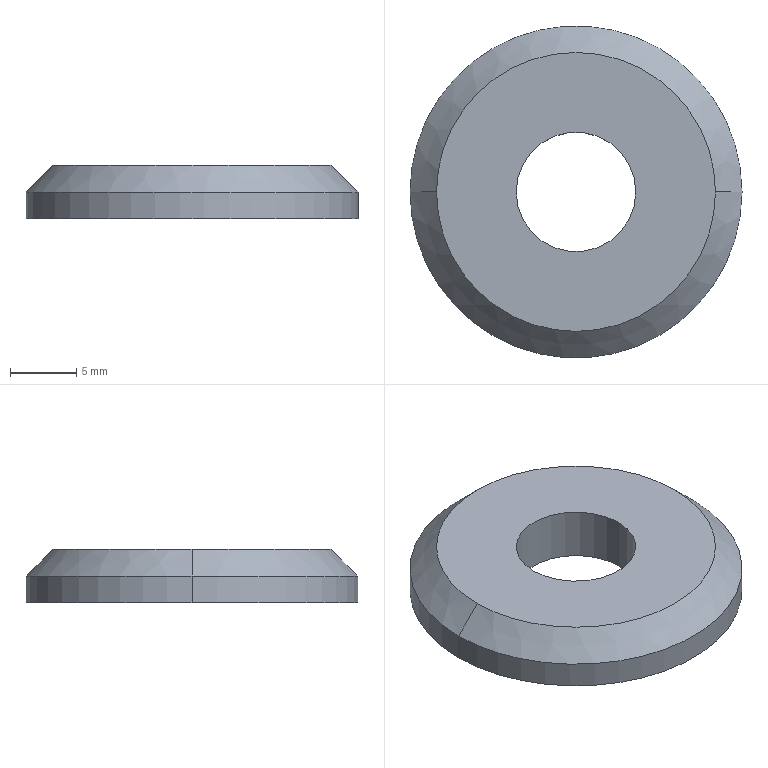Part | STEP file | Small washer | 1 solid | 8 faces | box 25 x 25 x 4 mm | volume 1560 mm3 | cylinder 4 | cone 2 | plane 2 | commonest cylinder face diameters 9 x2 25 x2
STEP:
#1=CARTESIAN_POINT('',(0.,0.,0.));
#2=DIRECTION('',(0.,0.,1.));
#3=DIRECTION('',(1.,0.,0.));
#4=AXIS2_PLACEMENT_3D('',#1,#2,#3);
#5=CARTESIAN_POINT('',(10.5,0.,4.));
#6=VERTEX_POINT('',#5);
#7=CARTESIAN_POINT('',(-10.5,0.,4.));
#8=VERTEX_POINT('',#7);
#9=CARTESIAN_POINT('',(0.,0.,4.));
#10=DIRECTION('',(0.,0.,1.));
#11=DIRECTION('',(1.,0.,0.));
#12=AXIS2_PLACEMENT_3D('',#9,#10,#11);
#13=CIRCLE('',#12,10.5);
#14=CARTESIAN_POINT('',(0.,0.,4.));
#15=DIRECTION('',(0.,0.,-1.));
#16=DIRECTION('',(-1.,0.,0.));
#17=AXIS2_PLACEMENT_3D('',#14,#15,#16);
#18=CONICAL_SURFACE('',#17,10.5,0.7854);
#19=CARTESIAN_POINT('',(3.142,0.));
#20=DIRECTION('',(-1.,0.));
#21=VECTOR('',#20,1.);
#22=LINE('',#19,#21);
#23=(GEOMETRIC_REPRESENTATION_CONTEXT(2)PARAMETRIC_REPRESENTATION_CONTEXT()REPRESENTATION_CONTEXT('',''));
#24=DEFINITIONAL_REPRESENTATION('',(#22),#23);
#25=PCURVE('',#18,#24);
#26=CARTESIAN_POINT('',(0.,0.,4.));
#27=DIRECTION('',(0.,0.,1.));
#28=DIRECTION('',(1.,0.,0.));
#29=AXIS2_PLACEMENT_3D('',#26,#27,#28);
#30=PLANE('',#29);
#31=CARTESIAN_POINT('',(0.,0.));
#32=DIRECTION('',(1.,0.));
#33=AXIS2_PLACEMENT_2D('',#31,#32);
#34=CIRCLE('',#33,10.5);
#35=(GEOMETRIC_REPRESENTATION_CONTEXT(2)PARAMETRIC_REPRESENTATION_CONTEXT()REPRESENTATION_CONTEXT('',''));
#36=DEFINITIONAL_REPRESENTATION('',(#34),#35);
#37=PCURVE('',#30,#36);
#38=SURFACE_CURVE('',#13,(#25,#37),.PCURVE_S1.);
#39=EDGE_CURVE('',#6,#8,#38,.T.);
#40=ORIENTED_EDGE('',*,*,#39,.F.);
#41=CARTESIAN_POINT('',(12.5,0.,2.));
#42=VERTEX_POINT('',#41);
#43=CARTESIAN_POINT('',(10.5,0.,4.));
#44=DIRECTION('',(0.7071,0.,-0.7071));
#45=VECTOR('',#44,1.);
#46=LINE('',#43,#45);
#47=CARTESIAN_POINT('',(3.142,0.));
#48=DIRECTION('',(0.,1.));
#49=VECTOR('',#48,1.);
#50=LINE('',#47,#49);
#51=(GEOMETRIC_REPRESENTATION_CONTEXT(2)PARAMETRIC_REPRESENTATION_CONTEXT()REPRESENTATION_CONTEXT('',''));
#52=DEFINITIONAL_REPRESENTATION('',(#50),#51);
#53=PCURVE('',#18,#52);
#54=CARTESIAN_POINT('',(0.,0.,4.));
#55=DIRECTION('',(0.,0.,-1.));
#56=DIRECTION('',(-1.,0.,0.));
#57=AXIS2_PLACEMENT_3D('',#54,#55,#56);
#58=CONICAL_SURFACE('',#57,10.5,0.7854);
#59=CARTESIAN_POINT('',(3.142,0.));
#60=DIRECTION('',(0.,1.));
#61=VECTOR('',#60,1.);
#62=LINE('',#59,#61);
#63=(GEOMETRIC_REPRESENTATION_CONTEXT(2)PARAMETRIC_REPRESENTATION_CONTEXT()REPRESENTATION_CONTEXT('',''));
#64=DEFINITIONAL_REPRESENTATION('',(#62),#63);
#65=PCURVE('',#58,#64);
#66=SURFACE_CURVE('',#46,(#53,#65),.PCURVE_S1.);
#67=EDGE_CURVE('',#6,#42,#66,.T.);
#68=ORIENTED_EDGE('',*,*,#67,.T.);
#69=CARTESIAN_POINT('',(-12.5,0.,2.));
#70=VERTEX_POINT('',#69);
#71=CARTESIAN_POINT('',(0.,0.,2.));
#72=DIRECTION('',(0.,0.,-1.));
#73=DIRECTION('',(1.,0.,0.));
#74=AXIS2_PLACEMENT_3D('',#71,#72,#73);
#75=CIRCLE('',#74,12.5);
#76=CARTESIAN_POINT('',(-3.142,2.));
#77=DIRECTION('',(1.,0.));
#78=VECTOR('',#77,1.);
#79=LINE('',#76,#78);
#80=(GEOMETRIC_REPRESENTATION_CONTEXT(2)PARAMETRIC_REPRESENTATION_CONTEXT()REPRESENTATION_CONTEXT('',''));
#81=DEFINITIONAL_REPRESENTATION('',(#79),#80);
#82=PCURVE('',#18,#81);
#83=CARTESIAN_POINT('',(0.,0.,4.));
#84=DIRECTION('',(0.,0.,-1.));
#85=DIRECTION('',(-1.,0.,0.));
#86=AXIS2_PLACEMENT_3D('',#83,#84,#85);
#87=CYLINDRICAL_SURFACE('',#86,12.5);
#88=CARTESIAN_POINT('',(-3.142,2.));
#89=DIRECTION('',(1.,0.));
#90=VECTOR('',#89,1.);
#91=LINE('',#88,#90);
#92=(GEOMETRIC_REPRESENTATION_CONTEXT(2)PARAMETRIC_REPRESENTATION_CONTEXT()REPRESENTATION_CONTEXT('',''));
#93=DEFINITIONAL_REPRESENTATION('',(#91),#92);
#94=PCURVE('',#87,#93);
#95=SURFACE_CURVE('',#75,(#82,#94),.PCURVE_S1.);
#96=EDGE_CURVE('',#70,#42,#95,.T.);
#97=ORIENTED_EDGE('',*,*,#96,.F.);
#98=CARTESIAN_POINT('',(-10.5,0.,4.));
#99=DIRECTION('',(-0.7071,0.,-0.7071));
#100=VECTOR('',#99,1.);
#101=LINE('',#98,#100);
#102=CARTESIAN_POINT('',(0.,0.));
#103=DIRECTION('',(0.,1.));
#104=VECTOR('',#103,1.);
#105=LINE('',#102,#104);
#106=(GEOMETRIC_REPRESENTATION_CONTEXT(2)PARAMETRIC_REPRESENTATION_CONTEXT()REPRESENTATION_CONTEXT('',''));
#107=DEFINITIONAL_REPRESENTATION('',(#105),#106);
#108=PCURVE('',#18,#107);
#109=CARTESIAN_POINT('',(6.283,0.));
#110=DIRECTION('',(0.,1.));
#111=VECTOR('',#110,1.);
#112=LINE('',#109,#111);
#113=(GEOMETRIC_REPRESENTATION_CONTEXT(2)PARAMETRIC_REPRESENTATION_CONTEXT()REPRESENTATION_CONTEXT('',''));
#114=DEFINITIONAL_REPRESENTATION('',(#112),#113);
#115=PCURVE('',#58,#114);
#116=SURFACE_CURVE('',#101,(#108,#115),.PCURVE_S1.);
#117=EDGE_CURVE('',#8,#70,#116,.T.);
#118=ORIENTED_EDGE('',*,*,#117,.F.);
#119=EDGE_LOOP('',(#40,#68,#97,#118));
#120=FACE_BOUND('',#119,.T.);
#121=ADVANCED_FACE('',(#120),#18,.T.);
#122=CARTESIAN_POINT('',(-4.5,0.,4.));
#123=VERTEX_POINT('',#122);
#124=CARTESIAN_POINT('',(-4.5,0.,0.));
#125=VERTEX_POINT('',#124);
#126=CARTESIAN_POINT('',(-4.5,0.,4.));
#127=DIRECTION('',(0.,0.,-1.));
#128=VECTOR('',#127,1.);
#129=LINE('',#126,#128);
#130=CARTESIAN_POINT('',(0.,0.,4.));
#131=DIRECTION('',(0.,0.,-1.));
#132=DIRECTION('',(-1.,0.,0.));
#133=AXIS2_PLACEMENT_3D('',#130,#131,#132);
#134=CYLINDRICAL_SURFACE('',#133,4.5);
#135=CARTESIAN_POINT('',(6.283,0.));
#136=DIRECTION('',(0.,1.));
#137=VECTOR('',#136,1.);
#138=LINE('',#135,#137);
#139=(GEOMETRIC_REPRESENTATION_CONTEXT(2)PARAMETRIC_REPRESENTATION_CONTEXT()REPRESENTATION_CONTEXT('',''));
#140=DEFINITIONAL_REPRESENTATION('',(#138),#139);
#141=PCURVE('',#134,#140);
#142=CARTESIAN_POINT('',(0.,0.,4.));
#143=DIRECTION('',(0.,0.,-1.));
#144=DIRECTION('',(-1.,0.,0.));
#145=AXIS2_PLACEMENT_3D('',#142,#143,#144);
#146=CYLINDRICAL_SURFACE('',#145,4.5);
#147=CARTESIAN_POINT('',(0.,0.));
#148=DIRECTION('',(0.,1.));
#149=VECTOR('',#148,1.);
#150=LINE('',#147,#149);
#151=(GEOMETRIC_REPRESENTATION_CONTEXT(2)PARAMETRIC_REPRESENTATION_CONTEXT()REPRESENTATION_CONTEXT('',''));
#152=DEFINITIONAL_REPRESENTATION('',(#150),#151);
#153=PCURVE('',#146,#152);
#154=SURFACE_CURVE('',#129,(#141,#153),.PCURVE_S1.);
#155=EDGE_CURVE('',#123,#125,#154,.T.);
#156=ORIENTED_EDGE('',*,*,#155,.T.);
#157=CARTESIAN_POINT('',(4.5,0.,0.));
#158=VERTEX_POINT('',#157);
#159=CARTESIAN_POINT('',(0.,0.,0.));
#160=DIRECTION('',(0.,0.,1.));
#161=DIRECTION('',(1.,0.,0.));
#162=AXIS2_PLACEMENT_3D('',#159,#160,#161);
#163=CIRCLE('',#162,4.5);
#164=CARTESIAN_POINT('',(9.425,4.));
#165=DIRECTION('',(-1.,0.));
#166=VECTOR('',#165,1.);
#167=LINE('',#164,#166);
#168=(GEOMETRIC_REPRESENTATION_CONTEXT(2)PARAMETRIC_REPRESENTATION_CONTEXT()REPRESENTATION_CONTEXT('',''));
#169=DEFINITIONAL_REPRESENTATION('',(#167),#168);
#170=PCURVE('',#134,#169);
#171=CARTESIAN_POINT('',(0.,0.,0.));
#172=DIRECTION('',(0.,0.,1.));
#173=DIRECTION('',(1.,0.,0.));
#174=AXIS2_PLACEMENT_3D('',#171,#172,#173);
#175=PLANE('',#174);
#176=CARTESIAN_POINT('',(0.,0.));
#177=DIRECTION('',(1.,0.));
#178=AXIS2_PLACEMENT_2D('',#176,#177);
#179=CIRCLE('',#178,4.5);
#180=(GEOMETRIC_REPRESENTATION_CONTEXT(2)PARAMETRIC_REPRESENTATION_CONTEXT()REPRESENTATION_CONTEXT('',''));
#181=DEFINITIONAL_REPRESENTATION('',(#179),#180);
#182=PCURVE('',#175,#181);
#183=SURFACE_CURVE('',#163,(#170,#182),.PCURVE_S1.);
#184=EDGE_CURVE('',#125,#158,#183,.T.);
#185=ORIENTED_EDGE('',*,*,#184,.T.);
#186=CARTESIAN_POINT('',(4.5,0.,4.));
#187=VERTEX_POINT('',#186);
#188=CARTESIAN_POINT('',(4.5,0.,4.));
#189=DIRECTION('',(0.,0.,-1.));
#190=VECTOR('',#189,1.);
#191=LINE('',#188,#190);
#192=CARTESIAN_POINT('',(3.142,0.));
#193=DIRECTION('',(0.,1.));
#194=VECTOR('',#193,1.);
#195=LINE('',#192,#194);
#196=(GEOMETRIC_REPRESENTATION_CONTEXT(2)PARAMETRIC_REPRESENTATION_CONTEXT()REPRESENTATION_CONTEXT('',''));
#197=DEFINITIONAL_REPRESENTATION('',(#195),#196);
#198=PCURVE('',#134,#197);
#199=CARTESIAN_POINT('',(3.142,0.));
#200=DIRECTION('',(0.,1.));
#201=VECTOR('',#200,1.);
#202=LINE('',#199,#201);
#203=(GEOMETRIC_REPRESENTATION_CONTEXT(2)PARAMETRIC_REPRESENTATION_CONTEXT()REPRESENTATION_CONTEXT('',''));
#204=DEFINITIONAL_REPRESENTATION('',(#202),#203);
#205=PCURVE('',#146,#204);
#206=SURFACE_CURVE('',#191,(#198,#205),.PCURVE_S1.);
#207=EDGE_CURVE('',#187,#158,#206,.T.);
#208=ORIENTED_EDGE('',*,*,#207,.F.);
#209=CARTESIAN_POINT('',(0.,0.,4.));
#210=DIRECTION('',(0.,0.,1.));
#211=DIRECTION('',(1.,0.,0.));
#212=AXIS2_PLACEMENT_3D('',#209,#210,#211);
#213=CIRCLE('',#212,4.5);
#214=CARTESIAN_POINT('',(9.425,0.));
#215=DIRECTION('',(-1.,0.));
#216=VECTOR('',#215,1.);
#217=LINE('',#214,#216);
#218=(GEOMETRIC_REPRESENTATION_CONTEXT(2)PARAMETRIC_REPRESENTATION_CONTEXT()REPRESENTATION_CONTEXT('',''));
#219=DEFINITIONAL_REPRESENTATION('',(#217),#218);
#220=PCURVE('',#134,#219);
#221=CARTESIAN_POINT('',(0.,0.));
#222=DIRECTION('',(1.,0.));
#223=AXIS2_PLACEMENT_2D('',#221,#222);
#224=CIRCLE('',#223,4.5);
#225=(GEOMETRIC_REPRESENTATION_CONTEXT(2)PARAMETRIC_REPRESENTATION_CONTEXT()REPRESENTATION_CONTEXT('',''));
#226=DEFINITIONAL_REPRESENTATION('',(#224),#225);
#227=PCURVE('',#30,#226);
#228=SURFACE_CURVE('',#213,(#220,#227),.PCURVE_S1.);
#229=EDGE_CURVE('',#123,#187,#228,.T.);
#230=ORIENTED_EDGE('',*,*,#229,.F.);
#231=EDGE_LOOP('',(#156,#185,#208,#230));
#232=FACE_BOUND('',#231,.F.);
#233=ADVANCED_FACE('',(#232),#134,.F.);
#234=ORIENTED_EDGE('',*,*,#96,.T.);
#235=CARTESIAN_POINT('',(12.5,0.,0.));
#236=VERTEX_POINT('',#235);
#237=CARTESIAN_POINT('',(12.5,0.,4.));
#238=DIRECTION('',(0.,0.,-1.));
#239=VECTOR('',#238,1.);
#240=LINE('',#237,#239);
#241=CARTESIAN_POINT('',(3.142,0.));
#242=DIRECTION('',(0.,1.));
#243=VECTOR('',#242,1.);
#244=LINE('',#241,#243);
#245=(GEOMETRIC_REPRESENTATION_CONTEXT(2)PARAMETRIC_REPRESENTATION_CONTEXT()REPRESENTATION_CONTEXT('',''));
#246=DEFINITIONAL_REPRESENTATION('',(#244),#245);
#247=PCURVE('',#87,#246);
#248=CARTESIAN_POINT('',(0.,0.,4.));
#249=DIRECTION('',(0.,0.,-1.));
#250=DIRECTION('',(-1.,0.,0.));
#251=AXIS2_PLACEMENT_3D('',#248,#249,#250);
#252=CYLINDRICAL_SURFACE('',#251,12.5);
#253=CARTESIAN_POINT('',(3.142,0.));
#254=DIRECTION('',(0.,1.));
#255=VECTOR('',#254,1.);
#256=LINE('',#253,#255);
#257=(GEOMETRIC_REPRESENTATION_CONTEXT(2)PARAMETRIC_REPRESENTATION_CONTEXT()REPRESENTATION_CONTEXT('',''));
#258=DEFINITIONAL_REPRESENTATION('',(#256),#257);
#259=PCURVE('',#252,#258);
#260=SURFACE_CURVE('',#240,(#247,#259),.PCURVE_S1.);
#261=EDGE_CURVE('',#42,#236,#260,.T.);
#262=ORIENTED_EDGE('',*,*,#261,.T.);
#263=CARTESIAN_POINT('',(-12.5,0.,0.));
#264=VERTEX_POINT('',#263);
#265=CARTESIAN_POINT('',(0.,0.,0.));
#266=DIRECTION('',(0.,0.,1.));
#267=DIRECTION('',(1.,0.,0.));
#268=AXIS2_PLACEMENT_3D('',#265,#266,#267);
#269=CIRCLE('',#268,12.5);
#270=CARTESIAN_POINT('',(3.142,4.));
#271=DIRECTION('',(-1.,0.));
#272=VECTOR('',#271,1.);
#273=LINE('',#270,#272);
#274=(GEOMETRIC_REPRESENTATION_CONTEXT(2)PARAMETRIC_REPRESENTATION_CONTEXT()REPRESENTATION_CONTEXT('',''));
#275=DEFINITIONAL_REPRESENTATION('',(#273),#274);
#276=PCURVE('',#87,#275);
#277=CARTESIAN_POINT('',(0.,0.));
#278=DIRECTION('',(1.,0.));
#279=AXIS2_PLACEMENT_2D('',#277,#278);
#280=CIRCLE('',#279,12.5);
#281=(GEOMETRIC_REPRESENTATION_CONTEXT(2)PARAMETRIC_REPRESENTATION_CONTEXT()REPRESENTATION_CONTEXT('',''));
#282=DEFINITIONAL_REPRESENTATION('',(#280),#281);
#283=PCURVE('',#175,#282);
#284=SURFACE_CURVE('',#269,(#276,#283),.PCURVE_S1.);
#285=EDGE_CURVE('',#236,#264,#284,.T.);
#286=ORIENTED_EDGE('',*,*,#285,.T.);
#287=CARTESIAN_POINT('',(-12.5,0.,4.));
#288=DIRECTION('',(0.,0.,-1.));
#289=VECTOR('',#288,1.);
#290=LINE('',#287,#289);
#291=CARTESIAN_POINT('',(0.,0.));
#292=DIRECTION('',(0.,1.));
#293=VECTOR('',#292,1.);
#294=LINE('',#291,#293);
#295=(GEOMETRIC_REPRESENTATION_CONTEXT(2)PARAMETRIC_REPRESENTATION_CONTEXT()REPRESENTATION_CONTEXT('',''));
#296=DEFINITIONAL_REPRESENTATION('',(#294),#295);
#297=PCURVE('',#87,#296);
#298=CARTESIAN_POINT('',(6.283,0.));
#299=DIRECTION('',(0.,1.));
#300=VECTOR('',#299,1.);
#301=LINE('',#298,#300);
#302=(GEOMETRIC_REPRESENTATION_CONTEXT(2)PARAMETRIC_REPRESENTATION_CONTEXT()REPRESENTATION_CONTEXT('',''));
#303=DEFINITIONAL_REPRESENTATION('',(#301),#302);
#304=PCURVE('',#252,#303);
#305=SURFACE_CURVE('',#290,(#297,#304),.PCURVE_S1.);
#306=EDGE_CURVE('',#70,#264,#305,.T.);
#307=ORIENTED_EDGE('',*,*,#306,.F.);
#308=EDGE_LOOP('',(#234,#262,#286,#307));
#309=FACE_BOUND('',#308,.T.);
#310=ADVANCED_FACE('',(#309),#87,.T.);
#311=CARTESIAN_POINT('',(0.,0.,4.));
#312=DIRECTION('',(0.,0.,1.));
#313=DIRECTION('',(1.,0.,0.));
#314=AXIS2_PLACEMENT_3D('',#311,#312,#313);
#315=CIRCLE('',#314,10.5);
#316=CARTESIAN_POINT('',(0.,0.));
#317=DIRECTION('',(1.,0.));
#318=AXIS2_PLACEMENT_2D('',#316,#317);
#319=CIRCLE('',#318,10.5);
#320=(GEOMETRIC_REPRESENTATION_CONTEXT(2)PARAMETRIC_REPRESENTATION_CONTEXT()REPRESENTATION_CONTEXT('',''));
#321=DEFINITIONAL_REPRESENTATION('',(#319),#320);
#322=PCURVE('',#30,#321);
#323=CARTESIAN_POINT('',(9.425,0.));
#324=DIRECTION('',(-1.,0.));
#325=VECTOR('',#324,1.);
#326=LINE('',#323,#325);
#327=(GEOMETRIC_REPRESENTATION_CONTEXT(2)PARAMETRIC_REPRESENTATION_CONTEXT()REPRESENTATION_CONTEXT('',''));
#328=DEFINITIONAL_REPRESENTATION('',(#326),#327);
#329=PCURVE('',#58,#328);
#330=SURFACE_CURVE('',#315,(#322,#329),.PCURVE_S1.);
#331=EDGE_CURVE('',#8,#6,#330,.T.);
#332=ORIENTED_EDGE('',*,*,#331,.T.);
#333=ORIENTED_EDGE('',*,*,#39,.T.);
#334=EDGE_LOOP('',(#332,#333));
#335=FACE_BOUND('',#334,.T.);
#336=ORIENTED_EDGE('',*,*,#229,.F.);
#337=CARTESIAN_POINT('',(0.,0.,4.));
#338=DIRECTION('',(0.,0.,1.));
#339=DIRECTION('',(1.,0.,0.));
#340=AXIS2_PLACEMENT_3D('',#337,#338,#339);
#341=CIRCLE('',#340,4.5);
#342=CARTESIAN_POINT('',(0.,0.));
#343=DIRECTION('',(1.,0.));
#344=AXIS2_PLACEMENT_2D('',#342,#343);
#345=CIRCLE('',#344,4.5);
#346=(GEOMETRIC_REPRESENTATION_CONTEXT(2)PARAMETRIC_REPRESENTATION_CONTEXT()REPRESENTATION_CONTEXT('',''));
#347=DEFINITIONAL_REPRESENTATION('',(#345),#346);
#348=PCURVE('',#30,#347);
#349=CARTESIAN_POINT('',(3.142,0.));
#350=DIRECTION('',(-1.,0.));
#351=VECTOR('',#350,1.);
#352=LINE('',#349,#351);
#353=(GEOMETRIC_REPRESENTATION_CONTEXT(2)PARAMETRIC_REPRESENTATION_CONTEXT()REPRESENTATION_CONTEXT('',''));
#354=DEFINITIONAL_REPRESENTATION('',(#352),#353);
#355=PCURVE('',#146,#354);
#356=SURFACE_CURVE('',#341,(#348,#355),.PCURVE_S1.);
#357=EDGE_CURVE('',#187,#123,#356,.T.);
#358=ORIENTED_EDGE('',*,*,#357,.F.);
#359=EDGE_LOOP('',(#336,#358));
#360=FACE_BOUND('',#359,.T.);
#361=ADVANCED_FACE('',(#335,#360),#30,.T.);
#362=CARTESIAN_POINT('',(0.,0.,0.));
#363=DIRECTION('',(0.,0.,1.));
#364=DIRECTION('',(1.,0.,0.));
#365=AXIS2_PLACEMENT_3D('',#362,#363,#364);
#366=CIRCLE('',#365,12.5);
#367=CARTESIAN_POINT('',(0.,0.));
#368=DIRECTION('',(1.,0.));
#369=AXIS2_PLACEMENT_2D('',#367,#368);
#370=CIRCLE('',#369,12.5);
#371=(GEOMETRIC_REPRESENTATION_CONTEXT(2)PARAMETRIC_REPRESENTATION_CONTEXT()REPRESENTATION_CONTEXT('',''));
#372=DEFINITIONAL_REPRESENTATION('',(#370),#371);
#373=PCURVE('',#175,#372);
#374=CARTESIAN_POINT('',(9.425,4.));
#375=DIRECTION('',(-1.,0.));
#376=VECTOR('',#375,1.);
#377=LINE('',#374,#376);
#378=(GEOMETRIC_REPRESENTATION_CONTEXT(2)PARAMETRIC_REPRESENTATION_CONTEXT()REPRESENTATION_CONTEXT('',''));
#379=DEFINITIONAL_REPRESENTATION('',(#377),#378);
#380=PCURVE('',#252,#379);
#381=SURFACE_CURVE('',#366,(#373,#380),.PCURVE_S1.);
#382=EDGE_CURVE('',#264,#236,#381,.T.);
#383=ORIENTED_EDGE('',*,*,#382,.F.);
#384=ORIENTED_EDGE('',*,*,#285,.F.);
#385=EDGE_LOOP('',(#383,#384));
#386=FACE_BOUND('',#385,.T.);
#387=ORIENTED_EDGE('',*,*,#184,.T.);
#388=CARTESIAN_POINT('',(0.,0.,0.));
#389=DIRECTION('',(0.,0.,1.));
#390=DIRECTION('',(1.,0.,0.));
#391=AXIS2_PLACEMENT_3D('',#388,#389,#390);
#392=CIRCLE('',#391,4.5);
#393=CARTESIAN_POINT('',(0.,0.));
#394=DIRECTION('',(1.,0.));
#395=AXIS2_PLACEMENT_2D('',#393,#394);
#396=CIRCLE('',#395,4.5);
#397=(GEOMETRIC_REPRESENTATION_CONTEXT(2)PARAMETRIC_REPRESENTATION_CONTEXT()REPRESENTATION_CONTEXT('',''));
#398=DEFINITIONAL_REPRESENTATION('',(#396),#397);
#399=PCURVE('',#175,#398);
#400=CARTESIAN_POINT('',(3.142,4.));
#401=DIRECTION('',(-1.,0.));
#402=VECTOR('',#401,1.);
#403=LINE('',#400,#402);
#404=(GEOMETRIC_REPRESENTATION_CONTEXT(2)PARAMETRIC_REPRESENTATION_CONTEXT()REPRESENTATION_CONTEXT('',''));
#405=DEFINITIONAL_REPRESENTATION('',(#403),#404);
#406=PCURVE('',#146,#405);
#407=SURFACE_CURVE('',#392,(#399,#406),.PCURVE_S1.);
#408=EDGE_CURVE('',#158,#125,#407,.T.);
#409=ORIENTED_EDGE('',*,*,#408,.T.);
#410=EDGE_LOOP('',(#387,#409));
#411=FACE_BOUND('',#410,.T.);
#412=ADVANCED_FACE('',(#386,#411),#175,.F.);
#413=ORIENTED_EDGE('',*,*,#261,.F.);
#414=CARTESIAN_POINT('',(0.,0.,2.));
#415=DIRECTION('',(0.,0.,-1.));
#416=DIRECTION('',(1.,0.,0.));
#417=AXIS2_PLACEMENT_3D('',#414,#415,#416);
#418=CIRCLE('',#417,12.5);
#419=CARTESIAN_POINT('',(3.142,2.));
#420=DIRECTION('',(1.,0.));
#421=VECTOR('',#420,1.);
#422=LINE('',#419,#421);
#423=(GEOMETRIC_REPRESENTATION_CONTEXT(2)PARAMETRIC_REPRESENTATION_CONTEXT()REPRESENTATION_CONTEXT('',''));
#424=DEFINITIONAL_REPRESENTATION('',(#422),#423);
#425=PCURVE('',#252,#424);
#426=CARTESIAN_POINT('',(3.142,2.));
#427=DIRECTION('',(1.,0.));
#428=VECTOR('',#427,1.);
#429=LINE('',#426,#428);
#430=(GEOMETRIC_REPRESENTATION_CONTEXT(2)PARAMETRIC_REPRESENTATION_CONTEXT()REPRESENTATION_CONTEXT('',''));
#431=DEFINITIONAL_REPRESENTATION('',(#429),#430);
#432=PCURVE('',#58,#431);
#433=SURFACE_CURVE('',#418,(#425,#432),.PCURVE_S1.);
#434=EDGE_CURVE('',#42,#70,#433,.T.);
#435=ORIENTED_EDGE('',*,*,#434,.T.);
#436=ORIENTED_EDGE('',*,*,#306,.T.);
#437=ORIENTED_EDGE('',*,*,#382,.T.);
#438=EDGE_LOOP('',(#413,#435,#436,#437));
#439=FACE_BOUND('',#438,.T.);
#440=ADVANCED_FACE('',(#439),#252,.T.);
#441=ORIENTED_EDGE('',*,*,#408,.T.);
#442=ORIENTED_EDGE('',*,*,#155,.F.);
#443=ORIENTED_EDGE('',*,*,#357,.F.);
#444=ORIENTED_EDGE('',*,*,#207,.T.);
#445=EDGE_LOOP('',(#441,#442,#443,#444));
#446=FACE_BOUND('',#445,.F.);
#447=ADVANCED_FACE('',(#446),#146,.F.);
#448=ORIENTED_EDGE('',*,*,#67,.F.);
#449=ORIENTED_EDGE('',*,*,#331,.F.);
#450=ORIENTED_EDGE('',*,*,#117,.T.);
#451=ORIENTED_EDGE('',*,*,#434,.F.);
#452=EDGE_LOOP('',(#448,#449,#450,#451));
#453=FACE_BOUND('',#452,.T.);
#454=ADVANCED_FACE('',(#453),#58,.T.);
#455=CLOSED_SHELL('',(#121,#233,#310,#361,#412,#440,#447,#454));
#456=MANIFOLD_SOLID_BREP('',#455);
#457=(LENGTH_UNIT()NAMED_UNIT(*)SI_UNIT(.MILLI.,.METRE.));
#458=UNCERTAINTY_MEASURE_WITH_UNIT(LENGTH_MEASURE(0.0000001),#457,'','');
#459=(NAMED_UNIT(*)PLANE_ANGLE_UNIT()SI_UNIT($,.RADIAN.));
#460=(NAMED_UNIT(*)SI_UNIT($,.STERADIAN.)SOLID_ANGLE_UNIT());
#461=(GEOMETRIC_REPRESENTATION_CONTEXT(3)GLOBAL_UNCERTAINTY_ASSIGNED_CONTEXT((#458))GLOBAL_UNIT_ASSIGNED_CONTEXT((#457,#459,#460))REPRESENTATION_CONTEXT('',''));
#462=ADVANCED_BREP_SHAPE_REPRESENTATION('',(#4,#456),#461);